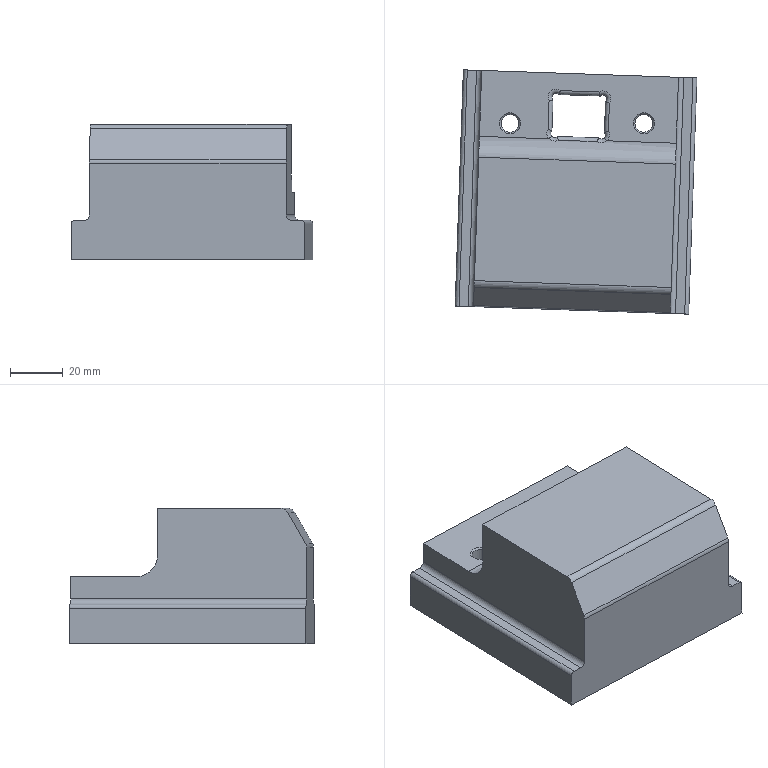Part | NX | features DIE-76 2 | 1 solid | 53 faces | box 92.086 x 93.051 x 51.5 mm | volume 284897 mm3 | plane 22 | cylinder 22 | torus 4 | cone 3 | spline 2 | commonest cylinder face diameters 3 x10 6 x6 4 x2 6.8 x2 6.806 x1 16 x1